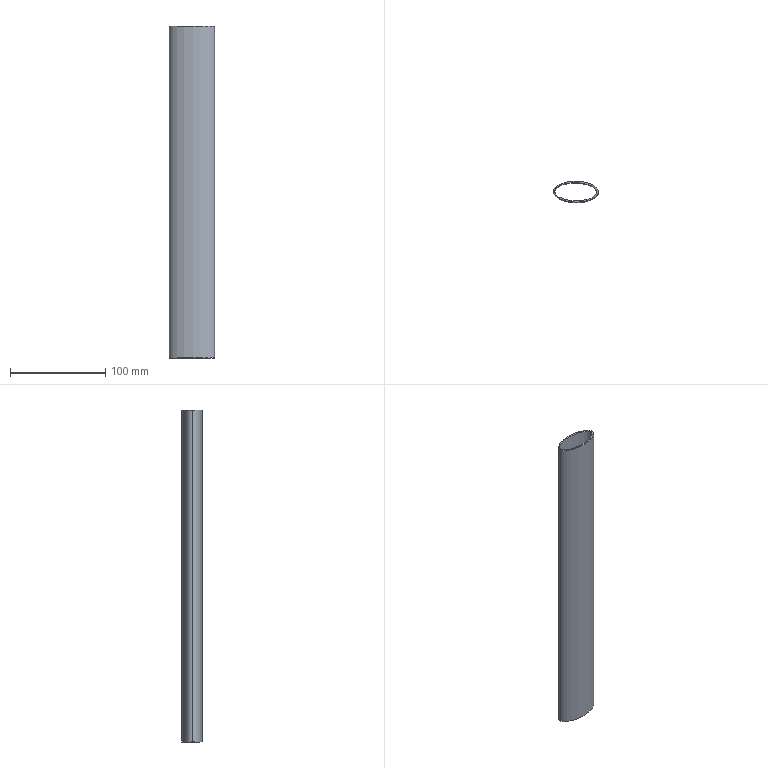Part | SolidWorks | features Extrusion 1 | 1 solid | 6 faces | box 47.25 x 22 x 348 mm | volume 56835 mm3 | spline 4 | plane 2
STEP:
#1=CARTESIAN_POINT('',(-22.094,38.091,15.874));
#2=VERTEX_POINT('',#1);
#3=CARTESIAN_POINT('',(-20.372,38.066,15.874));
#4=VERTEX_POINT('',#3);
#5=CARTESIAN_POINT('',(-22.094,38.091,15.874));
#6=CARTESIAN_POINT('',(-22.083,38.839,15.874));
#7=CARTESIAN_POINT('',(-20.362,38.815,15.874));
#8=CARTESIAN_POINT('',(-20.372,38.066,15.874));
#9=(BOUNDED_CURVE()B_SPLINE_CURVE(3,(#5,#6,#7,#8),.UNSPECIFIED.,.F.,.F.)B_SPLINE_CURVE_WITH_KNOTS((4,4),(3.142,6.283),.UNSPECIFIED.)CURVE()GEOMETRIC_REPRESENTATION_ITEM()RATIONAL_B_SPLINE_CURVE((1.,0.3333,0.3333,1.))REPRESENTATION_ITEM(''));
#10=EDGE_CURVE('',#2,#4,#9,.T.);
#11=ORIENTED_EDGE('',*,*,#10,.F.);
#12=CARTESIAN_POINT('',(-22.094,38.091,2.173));
#13=VERTEX_POINT('',#12);
#14=CARTESIAN_POINT('',(-22.094,38.091,15.874));
#15=DIRECTION('',(0.,0.,-1.));
#16=VECTOR('',#15,39.37);
#17=LINE('',#14,#16);
#18=EDGE_CURVE('',#2,#13,#17,.T.);
#19=ORIENTED_EDGE('',*,*,#18,.T.);
#20=CARTESIAN_POINT('',(-20.372,38.066,2.173));
#21=VERTEX_POINT('',#20);
#22=CARTESIAN_POINT('',(-22.094,38.091,2.173));
#23=CARTESIAN_POINT('',(-22.083,38.839,2.173));
#24=CARTESIAN_POINT('',(-20.362,38.815,2.173));
#25=CARTESIAN_POINT('',(-20.372,38.066,2.173));
#26=(BOUNDED_CURVE()B_SPLINE_CURVE(3,(#22,#23,#24,#25),.UNSPECIFIED.,.F.,.F.)B_SPLINE_CURVE_WITH_KNOTS((4,4),(3.142,6.283),.UNSPECIFIED.)CURVE()GEOMETRIC_REPRESENTATION_ITEM()RATIONAL_B_SPLINE_CURVE((1.,0.3333,0.3333,1.))REPRESENTATION_ITEM(''));
#27=EDGE_CURVE('',#13,#21,#26,.T.);
#28=ORIENTED_EDGE('',*,*,#27,.T.);
#29=CARTESIAN_POINT('',(-20.372,38.066,15.874));
#30=DIRECTION('',(0.,0.,-1.));
#31=VECTOR('',#30,39.37);
#32=LINE('',#29,#31);
#33=EDGE_CURVE('',#4,#21,#32,.T.);
#34=ORIENTED_EDGE('',*,*,#33,.F.);
#35=EDGE_LOOP('',(#11,#19,#28,#34));
#36=FACE_OUTER_BOUND('',#35,.T.);
#37=CARTESIAN_POINT('',(-22.094,38.091,15.874));
#38=CARTESIAN_POINT('',(-22.094,38.091,2.173));
#39=CARTESIAN_POINT('',(-22.083,38.839,15.874));
#40=CARTESIAN_POINT('',(-22.083,38.839,2.173));
#41=CARTESIAN_POINT('',(-20.362,38.815,15.874));
#42=CARTESIAN_POINT('',(-20.362,38.815,2.173));
#43=CARTESIAN_POINT('',(-20.372,38.066,15.874));
#44=CARTESIAN_POINT('',(-20.372,38.066,2.173));
#45=(BOUNDED_SURFACE()B_SPLINE_SURFACE(3,1,((#37,#38),(#39,#40),(#41,#42),(#43,#44)),.UNSPECIFIED.,.F.,.F.,.T.)B_SPLINE_SURFACE_WITH_KNOTS((4,4),(2,2),(0.,1.),(0.,1.),.UNSPECIFIED.)GEOMETRIC_REPRESENTATION_ITEM()RATIONAL_B_SPLINE_SURFACE(((1.,1.),(0.3333,0.3333),(0.3333,0.3333),(1.,1.)))REPRESENTATION_ITEM('')SURFACE());
#46=ADVANCED_FACE('',(#36),#45,.F.);
#47=CARTESIAN_POINT('',(-20.29,38.079,15.874));
#48=VERTEX_POINT('',#47);
#49=CARTESIAN_POINT('',(-22.151,38.079,15.874));
#50=VERTEX_POINT('',#49);
#51=CARTESIAN_POINT('',(-20.29,38.079,15.874));
#52=CARTESIAN_POINT('',(-20.29,37.213,15.874));
#53=CARTESIAN_POINT('',(-22.151,37.213,15.874));
#54=CARTESIAN_POINT('',(-22.151,38.079,15.874));
#55=(BOUNDED_CURVE()B_SPLINE_CURVE(3,(#51,#52,#53,#54),.UNSPECIFIED.,.F.,.F.)B_SPLINE_CURVE_WITH_KNOTS((4,4),(0.,3.142),.UNSPECIFIED.)CURVE()GEOMETRIC_REPRESENTATION_ITEM()RATIONAL_B_SPLINE_CURVE((1.,0.3333,0.3333,1.))REPRESENTATION_ITEM(''));
#56=EDGE_CURVE('',#48,#50,#55,.T.);
#57=ORIENTED_EDGE('',*,*,#56,.T.);
#58=CARTESIAN_POINT('',(-22.151,38.079,2.173));
#59=VERTEX_POINT('',#58);
#60=CARTESIAN_POINT('',(-22.151,38.079,15.874));
#61=DIRECTION('',(0.,0.,-1.));
#62=VECTOR('',#61,39.37);
#63=LINE('',#60,#62);
#64=EDGE_CURVE('',#50,#59,#63,.T.);
#65=ORIENTED_EDGE('',*,*,#64,.T.);
#66=CARTESIAN_POINT('',(-20.29,38.079,2.173));
#67=VERTEX_POINT('',#66);
#68=CARTESIAN_POINT('',(-20.29,38.079,2.173));
#69=CARTESIAN_POINT('',(-20.29,37.213,2.173));
#70=CARTESIAN_POINT('',(-22.151,37.213,2.173));
#71=CARTESIAN_POINT('',(-22.151,38.079,2.173));
#72=(BOUNDED_CURVE()B_SPLINE_CURVE(3,(#68,#69,#70,#71),.UNSPECIFIED.,.F.,.F.)B_SPLINE_CURVE_WITH_KNOTS((4,4),(0.,3.142),.UNSPECIFIED.)CURVE()GEOMETRIC_REPRESENTATION_ITEM()RATIONAL_B_SPLINE_CURVE((1.,0.3333,0.3333,1.))REPRESENTATION_ITEM(''));
#73=EDGE_CURVE('',#67,#59,#72,.T.);
#74=ORIENTED_EDGE('',*,*,#73,.F.);
#75=CARTESIAN_POINT('',(-20.29,38.079,15.874));
#76=DIRECTION('',(0.,0.,-1.));
#77=VECTOR('',#76,39.37);
#78=LINE('',#75,#77);
#79=EDGE_CURVE('',#48,#67,#78,.T.);
#80=ORIENTED_EDGE('',*,*,#79,.F.);
#81=EDGE_LOOP('',(#57,#65,#74,#80));
#82=FACE_OUTER_BOUND('',#81,.T.);
#83=CARTESIAN_POINT('',(-20.29,38.079,15.874));
#84=CARTESIAN_POINT('',(-20.29,38.079,2.173));
#85=CARTESIAN_POINT('',(-20.29,37.213,15.874));
#86=CARTESIAN_POINT('',(-20.29,37.213,2.173));
#87=CARTESIAN_POINT('',(-22.151,37.213,15.874));
#88=CARTESIAN_POINT('',(-22.151,37.213,2.173));
#89=CARTESIAN_POINT('',(-22.151,38.079,15.874));
#90=CARTESIAN_POINT('',(-22.151,38.079,2.173));
#91=(BOUNDED_SURFACE()B_SPLINE_SURFACE(3,1,((#83,#84),(#85,#86),(#87,#88),(#89,#90)),.UNSPECIFIED.,.F.,.F.,.F.)B_SPLINE_SURFACE_WITH_KNOTS((4,4),(2,2),(0.,1.),(0.,1.),.UNSPECIFIED.)GEOMETRIC_REPRESENTATION_ITEM()RATIONAL_B_SPLINE_SURFACE(((1.,1.),(0.3333,0.3333),(0.3333,0.3333),(1.,1.)))REPRESENTATION_ITEM('')SURFACE());
#92=ADVANCED_FACE('',(#82),#91,.T.);
#93=ORIENTED_EDGE('',*,*,#64,.F.);
#94=CARTESIAN_POINT('',(-22.151,38.079,15.874));
#95=CARTESIAN_POINT('',(-22.151,38.945,15.874));
#96=CARTESIAN_POINT('',(-20.29,38.945,15.874));
#97=CARTESIAN_POINT('',(-20.29,38.079,15.874));
#98=(BOUNDED_CURVE()B_SPLINE_CURVE(3,(#94,#95,#96,#97),.UNSPECIFIED.,.F.,.F.)B_SPLINE_CURVE_WITH_KNOTS((4,4),(3.142,6.283),.UNSPECIFIED.)CURVE()GEOMETRIC_REPRESENTATION_ITEM()RATIONAL_B_SPLINE_CURVE((1.,0.3333,0.3333,1.))REPRESENTATION_ITEM(''));
#99=EDGE_CURVE('',#50,#48,#98,.T.);
#100=ORIENTED_EDGE('',*,*,#99,.T.);
#101=ORIENTED_EDGE('',*,*,#79,.T.);
#102=CARTESIAN_POINT('',(-22.151,38.079,2.173));
#103=CARTESIAN_POINT('',(-22.151,38.945,2.173));
#104=CARTESIAN_POINT('',(-20.29,38.945,2.173));
#105=CARTESIAN_POINT('',(-20.29,38.079,2.173));
#106=(BOUNDED_CURVE()B_SPLINE_CURVE(3,(#102,#103,#104,#105),.UNSPECIFIED.,.F.,.F.)B_SPLINE_CURVE_WITH_KNOTS((4,4),(3.142,6.283),.UNSPECIFIED.)CURVE()GEOMETRIC_REPRESENTATION_ITEM()RATIONAL_B_SPLINE_CURVE((1.,0.3333,0.3333,1.))REPRESENTATION_ITEM(''));
#107=EDGE_CURVE('',#59,#67,#106,.T.);
#108=ORIENTED_EDGE('',*,*,#107,.F.);
#109=EDGE_LOOP('',(#93,#100,#101,#108));
#110=FACE_OUTER_BOUND('',#109,.T.);
#111=CARTESIAN_POINT('',(-22.151,38.079,15.874));
#112=CARTESIAN_POINT('',(-22.151,38.079,2.173));
#113=CARTESIAN_POINT('',(-22.151,38.945,15.874));
#114=CARTESIAN_POINT('',(-22.151,38.945,2.173));
#115=CARTESIAN_POINT('',(-20.29,38.945,15.874));
#116=CARTESIAN_POINT('',(-20.29,38.945,2.173));
#117=CARTESIAN_POINT('',(-20.29,38.079,15.874));
#118=CARTESIAN_POINT('',(-20.29,38.079,2.173));
#119=(BOUNDED_SURFACE()B_SPLINE_SURFACE(3,1,((#111,#112),(#113,#114),(#115,#116),(#117,#118)),.UNSPECIFIED.,.F.,.F.,.F.)B_SPLINE_SURFACE_WITH_KNOTS((4,4),(2,2),(0.,1.),(0.,1.),.UNSPECIFIED.)GEOMETRIC_REPRESENTATION_ITEM()RATIONAL_B_SPLINE_SURFACE(((1.,1.),(0.3333,0.3333),(0.3333,0.3333),(1.,1.)))REPRESENTATION_ITEM('')SURFACE());
#120=ADVANCED_FACE('',(#110),#119,.T.);
#121=CARTESIAN_POINT('',(-20.372,38.066,15.874));
#122=CARTESIAN_POINT('',(-20.383,37.318,15.874));
#123=CARTESIAN_POINT('',(-22.105,37.342,15.874));
#124=CARTESIAN_POINT('',(-22.094,38.091,15.874));
#125=(BOUNDED_CURVE()B_SPLINE_CURVE(3,(#121,#122,#123,#124),.UNSPECIFIED.,.F.,.F.)B_SPLINE_CURVE_WITH_KNOTS((4,4),(0.,3.142),.UNSPECIFIED.)CURVE()GEOMETRIC_REPRESENTATION_ITEM()RATIONAL_B_SPLINE_CURVE((1.,0.3333,0.3333,1.))REPRESENTATION_ITEM(''));
#126=EDGE_CURVE('',#4,#2,#125,.T.);
#127=ORIENTED_EDGE('',*,*,#126,.T.);
#128=ORIENTED_EDGE('',*,*,#10,.T.);
#129=EDGE_LOOP('',(#127,#128));
#130=FACE_BOUND('',#129,.T.);
#131=ORIENTED_EDGE('',*,*,#56,.F.);
#132=ORIENTED_EDGE('',*,*,#99,.F.);
#133=EDGE_LOOP('',(#131,#132));
#134=FACE_OUTER_BOUND('',#133,.T.);
#135=CARTESIAN_POINT('',(-21.22,38.079,15.874));
#136=DIRECTION('',(0.,0.,-1.));
#137=DIRECTION('',(0.,1.,0.));
#138=AXIS2_PLACEMENT_3D('',#135,#136,#137);
#139=PLANE('',#138);
#140=ADVANCED_FACE('',(#130,#134),#139,.F.);
#141=CARTESIAN_POINT('',(-20.372,38.066,2.173));
#142=CARTESIAN_POINT('',(-20.383,37.318,2.173));
#143=CARTESIAN_POINT('',(-22.105,37.342,2.173));
#144=CARTESIAN_POINT('',(-22.094,38.091,2.173));
#145=(BOUNDED_CURVE()B_SPLINE_CURVE(3,(#141,#142,#143,#144),.UNSPECIFIED.,.F.,.F.)B_SPLINE_CURVE_WITH_KNOTS((4,4),(0.,3.142),.UNSPECIFIED.)CURVE()GEOMETRIC_REPRESENTATION_ITEM()RATIONAL_B_SPLINE_CURVE((1.,0.3333,0.3333,1.))REPRESENTATION_ITEM(''));
#146=EDGE_CURVE('',#21,#13,#145,.T.);
#147=ORIENTED_EDGE('',*,*,#146,.F.);
#148=ORIENTED_EDGE('',*,*,#27,.F.);
#149=EDGE_LOOP('',(#147,#148));
#150=FACE_BOUND('',#149,.T.);
#151=ORIENTED_EDGE('',*,*,#73,.T.);
#152=ORIENTED_EDGE('',*,*,#107,.T.);
#153=EDGE_LOOP('',(#151,#152));
#154=FACE_OUTER_BOUND('',#153,.T.);
#155=CARTESIAN_POINT('',(-21.22,38.079,2.173));
#156=DIRECTION('',(0.,0.,-1.));
#157=DIRECTION('',(0.,1.,0.));
#158=AXIS2_PLACEMENT_3D('',#155,#156,#157);
#159=PLANE('',#158);
#160=ADVANCED_FACE('',(#150,#154),#159,.T.);
#161=ORIENTED_EDGE('',*,*,#18,.F.);
#162=ORIENTED_EDGE('',*,*,#126,.F.);
#163=ORIENTED_EDGE('',*,*,#33,.T.);
#164=ORIENTED_EDGE('',*,*,#146,.T.);
#165=EDGE_LOOP('',(#161,#162,#163,#164));
#166=FACE_OUTER_BOUND('',#165,.T.);
#167=CARTESIAN_POINT('',(-20.372,38.066,15.874));
#168=CARTESIAN_POINT('',(-20.372,38.066,2.173));
#169=CARTESIAN_POINT('',(-20.383,37.318,15.874));
#170=CARTESIAN_POINT('',(-20.383,37.318,2.173));
#171=CARTESIAN_POINT('',(-22.105,37.342,15.874));
#172=CARTESIAN_POINT('',(-22.105,37.342,2.173));
#173=CARTESIAN_POINT('',(-22.094,38.091,15.874));
#174=CARTESIAN_POINT('',(-22.094,38.091,2.173));
#175=(BOUNDED_SURFACE()B_SPLINE_SURFACE(3,1,((#167,#168),(#169,#170),(#171,#172),(#173,#174)),.UNSPECIFIED.,.F.,.F.,.F.)B_SPLINE_SURFACE_WITH_KNOTS((4,4),(2,2),(0.,1.),(0.,1.),.UNSPECIFIED.)GEOMETRIC_REPRESENTATION_ITEM()RATIONAL_B_SPLINE_SURFACE(((1.,1.),(0.3333,0.3333),(0.3333,0.3333),(1.,1.)))REPRESENTATION_ITEM('')SURFACE());
#176=ADVANCED_FACE('',(#166),#175,.F.);
#177=CLOSED_SHELL('',(#46,#92,#120,#140,#160,#176));
#178=MANIFOLD_SOLID_BREP('',#177);
#179=CARTESIAN_POINT('',(0.,0.,0.));
#180=DIRECTION('',(0.,0.,1.));
#181=DIRECTION('',(1.,0.,0.));
#182=AXIS2_PLACEMENT_3D('',#179,#180,#181);
#183=(LENGTH_UNIT()NAMED_UNIT(*)SI_UNIT($,.METRE.));
#184=LENGTH_MEASURE_WITH_UNIT(LENGTH_MEASURE(0.0254),#183);
#185=DIMENSIONAL_EXPONENTS(1.,0.,0.,0.,0.,0.,0.);
#186=(CONVERSION_BASED_UNIT('INCH',#184)LENGTH_UNIT()NAMED_UNIT(#185));
#187=UNCERTAINTY_MEASURE_WITH_UNIT(LENGTH_MEASURE(0.00001),#186,'','');
#188=(NAMED_UNIT(*)PLANE_ANGLE_UNIT()SI_UNIT($,.RADIAN.));
#189=(NAMED_UNIT(*)SI_UNIT($,.STERADIAN.)SOLID_ANGLE_UNIT());
#190=(GEOMETRIC_REPRESENTATION_CONTEXT(3)GLOBAL_UNCERTAINTY_ASSIGNED_CONTEXT((#187))GLOBAL_UNIT_ASSIGNED_CONTEXT((#186,#188,#189))REPRESENTATION_CONTEXT('',''));
#191=ADVANCED_BREP_SHAPE_REPRESENTATION('',(#178,#182),#190);